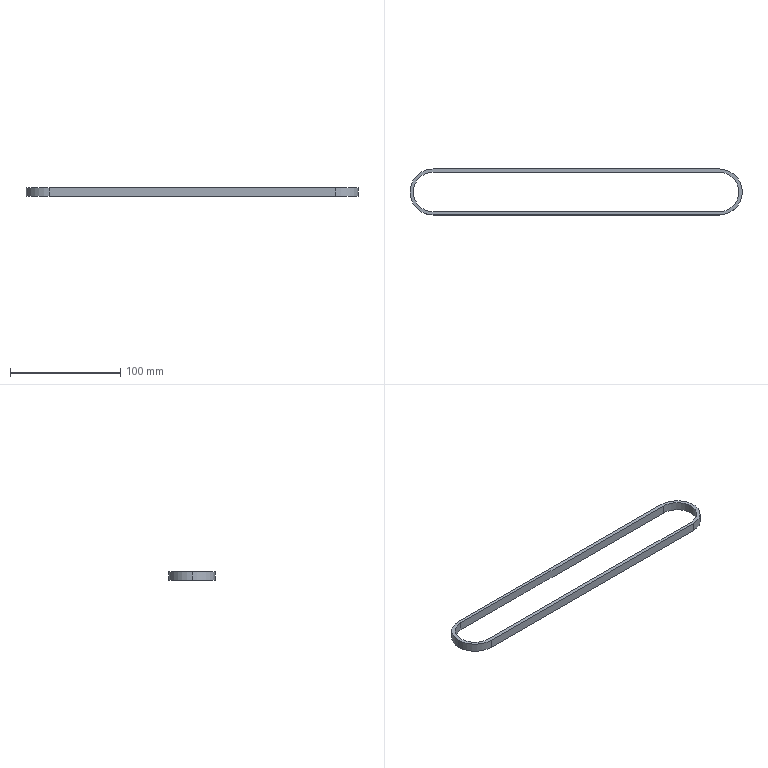Part | SolidWorks | features Extrusion 1, Shell 1 | 1 solid | 12 faces | box 301.8 x 41.8 x 7.9 mm | volume 15213 mm3 | cylinder 6 | plane 6 | commonest cylinder face diameters 35.8 x3 41.8 x3
STEP:
#1=CARTESIAN_POINT('',(-260.,17.9,7.9));
#2=VERTEX_POINT('',#1);
#3=CARTESIAN_POINT('',(-277.9,0.,7.9));
#4=VERTEX_POINT('',#3);
#5=CARTESIAN_POINT('',(-260.,0.,7.9));
#6=DIRECTION('',(0.,0.,1.));
#7=DIRECTION('',(1.,0.,0.));
#8=AXIS2_PLACEMENT_3D('',#5,#6,#7);
#9=CIRCLE('',#8,17.9);
#10=EDGE_CURVE('',#2,#4,#9,.T.);
#11=ORIENTED_EDGE('',*,*,#10,.T.);
#12=CARTESIAN_POINT('',(-277.9,0.,0.));
#13=VERTEX_POINT('',#12);
#14=CARTESIAN_POINT('',(-277.9,0.,7.9));
#15=DIRECTION('',(0.,0.,-1.));
#16=VECTOR('',#15,1000.);
#17=LINE('',#14,#16);
#18=EDGE_CURVE('',#4,#13,#17,.T.);
#19=ORIENTED_EDGE('',*,*,#18,.T.);
#20=CARTESIAN_POINT('',(-260.,17.9,0.));
#21=VERTEX_POINT('',#20);
#22=CARTESIAN_POINT('',(-260.,0.,0.));
#23=DIRECTION('',(0.,0.,1.));
#24=DIRECTION('',(1.,0.,0.));
#25=AXIS2_PLACEMENT_3D('',#22,#23,#24);
#26=CIRCLE('',#25,17.9);
#27=EDGE_CURVE('',#21,#13,#26,.T.);
#28=ORIENTED_EDGE('',*,*,#27,.F.);
#29=CARTESIAN_POINT('',(-260.,17.9,7.9));
#30=DIRECTION('',(0.,0.,-1.));
#31=VECTOR('',#30,1000.);
#32=LINE('',#29,#31);
#33=EDGE_CURVE('',#2,#21,#32,.T.);
#34=ORIENTED_EDGE('',*,*,#33,.F.);
#35=EDGE_LOOP('',(#11,#19,#28,#34));
#36=FACE_OUTER_BOUND('',#35,.T.);
#37=CARTESIAN_POINT('',(-260.,0.,7.9));
#38=DIRECTION('',(0.,0.,-1.));
#39=DIRECTION('',(-1.,0.,0.));
#40=AXIS2_PLACEMENT_3D('',#37,#38,#39);
#41=CYLINDRICAL_SURFACE('',#40,17.9);
#42=ADVANCED_FACE('',(#36),#41,.F.);
#43=CARTESIAN_POINT('',(-280.9,0.,7.9));
#44=VERTEX_POINT('',#43);
#45=CARTESIAN_POINT('',(-260.,-20.9,7.9));
#46=VERTEX_POINT('',#45);
#47=CARTESIAN_POINT('',(-260.,0.,7.9));
#48=DIRECTION('',(0.,0.,1.));
#49=DIRECTION('',(1.,0.,0.));
#50=AXIS2_PLACEMENT_3D('',#47,#48,#49);
#51=CIRCLE('',#50,20.9);
#52=EDGE_CURVE('',#44,#46,#51,.T.);
#53=ORIENTED_EDGE('',*,*,#52,.F.);
#54=CARTESIAN_POINT('',(-280.9,0.,0.));
#55=VERTEX_POINT('',#54);
#56=CARTESIAN_POINT('',(-280.9,0.,7.9));
#57=DIRECTION('',(0.,0.,-1.));
#58=VECTOR('',#57,1000.);
#59=LINE('',#56,#58);
#60=EDGE_CURVE('',#44,#55,#59,.T.);
#61=ORIENTED_EDGE('',*,*,#60,.T.);
#62=CARTESIAN_POINT('',(-260.,-20.9,0.));
#63=VERTEX_POINT('',#62);
#64=CARTESIAN_POINT('',(-260.,0.,0.));
#65=DIRECTION('',(0.,0.,1.));
#66=DIRECTION('',(1.,0.,0.));
#67=AXIS2_PLACEMENT_3D('',#64,#65,#66);
#68=CIRCLE('',#67,20.9);
#69=EDGE_CURVE('',#55,#63,#68,.T.);
#70=ORIENTED_EDGE('',*,*,#69,.T.);
#71=CARTESIAN_POINT('',(-260.,-20.9,7.9));
#72=DIRECTION('',(0.,0.,-1.));
#73=VECTOR('',#72,1000.);
#74=LINE('',#71,#73);
#75=EDGE_CURVE('',#46,#63,#74,.T.);
#76=ORIENTED_EDGE('',*,*,#75,.F.);
#77=EDGE_LOOP('',(#53,#61,#70,#76));
#78=FACE_OUTER_BOUND('',#77,.T.);
#79=CARTESIAN_POINT('',(-260.,0.,7.9));
#80=DIRECTION('',(0.,0.,-1.));
#81=DIRECTION('',(-1.,0.,0.));
#82=AXIS2_PLACEMENT_3D('',#79,#80,#81);
#83=CYLINDRICAL_SURFACE('',#82,20.9);
#84=ADVANCED_FACE('',(#78),#83,.T.);
#85=CARTESIAN_POINT('',(0.,-20.9,0.));
#86=VERTEX_POINT('',#85);
#87=CARTESIAN_POINT('',(0.,20.9,0.));
#88=VERTEX_POINT('',#87);
#89=CARTESIAN_POINT('',(0.,0.,0.));
#90=DIRECTION('',(0.,0.,1.));
#91=DIRECTION('',(1.,0.,0.));
#92=AXIS2_PLACEMENT_3D('',#89,#90,#91);
#93=CIRCLE('',#92,20.9);
#94=EDGE_CURVE('',#86,#88,#93,.T.);
#95=ORIENTED_EDGE('',*,*,#94,.T.);
#96=CARTESIAN_POINT('',(0.,20.9,7.9));
#97=VERTEX_POINT('',#96);
#98=CARTESIAN_POINT('',(0.,20.9,7.9));
#99=DIRECTION('',(0.,0.,-1.));
#100=VECTOR('',#99,1000.);
#101=LINE('',#98,#100);
#102=EDGE_CURVE('',#97,#88,#101,.T.);
#103=ORIENTED_EDGE('',*,*,#102,.F.);
#104=CARTESIAN_POINT('',(0.,-20.9,7.9));
#105=VERTEX_POINT('',#104);
#106=CARTESIAN_POINT('',(0.,0.,7.9));
#107=DIRECTION('',(0.,0.,1.));
#108=DIRECTION('',(1.,0.,0.));
#109=AXIS2_PLACEMENT_3D('',#106,#107,#108);
#110=CIRCLE('',#109,20.9);
#111=EDGE_CURVE('',#105,#97,#110,.T.);
#112=ORIENTED_EDGE('',*,*,#111,.F.);
#113=CARTESIAN_POINT('',(0.,-20.9,7.9));
#114=DIRECTION('',(0.,0.,-1.));
#115=VECTOR('',#114,1000.);
#116=LINE('',#113,#115);
#117=EDGE_CURVE('',#105,#86,#116,.T.);
#118=ORIENTED_EDGE('',*,*,#117,.T.);
#119=EDGE_LOOP('',(#95,#103,#112,#118));
#120=FACE_OUTER_BOUND('',#119,.T.);
#121=CARTESIAN_POINT('',(0.,0.,7.9));
#122=DIRECTION('',(0.,0.,-1.));
#123=DIRECTION('',(-1.,0.,0.));
#124=AXIS2_PLACEMENT_3D('',#121,#122,#123);
#125=CYLINDRICAL_SURFACE('',#124,20.9);
#126=ADVANCED_FACE('',(#120),#125,.T.);
#127=CARTESIAN_POINT('',(-260.,20.9,0.));
#128=VERTEX_POINT('',#127);
#129=CARTESIAN_POINT('',(0.,20.9,0.));
#130=DIRECTION('',(-1.,0.,0.));
#131=VECTOR('',#130,1000.);
#132=LINE('',#129,#131);
#133=EDGE_CURVE('',#88,#128,#132,.T.);
#134=ORIENTED_EDGE('',*,*,#133,.T.);
#135=CARTESIAN_POINT('',(-260.,20.9,7.9));
#136=VERTEX_POINT('',#135);
#137=CARTESIAN_POINT('',(-260.,20.9,7.9));
#138=DIRECTION('',(0.,0.,-1.));
#139=VECTOR('',#138,1000.);
#140=LINE('',#137,#139);
#141=EDGE_CURVE('',#136,#128,#140,.T.);
#142=ORIENTED_EDGE('',*,*,#141,.F.);
#143=CARTESIAN_POINT('',(0.,20.9,7.9));
#144=DIRECTION('',(-1.,0.,0.));
#145=VECTOR('',#144,1000.);
#146=LINE('',#143,#145);
#147=EDGE_CURVE('',#97,#136,#146,.T.);
#148=ORIENTED_EDGE('',*,*,#147,.F.);
#149=ORIENTED_EDGE('',*,*,#102,.T.);
#150=EDGE_LOOP('',(#134,#142,#148,#149));
#151=FACE_OUTER_BOUND('',#150,.T.);
#152=CARTESIAN_POINT('',(0.,20.9,7.9));
#153=DIRECTION('',(0.,-1.,0.));
#154=DIRECTION('',(0.,0.,-1.));
#155=AXIS2_PLACEMENT_3D('',#152,#153,#154);
#156=PLANE('',#155);
#157=ADVANCED_FACE('',(#151),#156,.F.);
#158=ORIENTED_EDGE('',*,*,#60,.F.);
#159=CARTESIAN_POINT('',(-260.,0.,7.9));
#160=DIRECTION('',(0.,0.,1.));
#161=DIRECTION('',(1.,0.,0.));
#162=AXIS2_PLACEMENT_3D('',#159,#160,#161);
#163=CIRCLE('',#162,20.9);
#164=EDGE_CURVE('',#136,#44,#163,.T.);
#165=ORIENTED_EDGE('',*,*,#164,.F.);
#166=ORIENTED_EDGE('',*,*,#141,.T.);
#167=CARTESIAN_POINT('',(-260.,0.,0.));
#168=DIRECTION('',(0.,0.,1.));
#169=DIRECTION('',(1.,0.,0.));
#170=AXIS2_PLACEMENT_3D('',#167,#168,#169);
#171=CIRCLE('',#170,20.9);
#172=EDGE_CURVE('',#128,#55,#171,.T.);
#173=ORIENTED_EDGE('',*,*,#172,.T.);
#174=EDGE_LOOP('',(#158,#165,#166,#173));
#175=FACE_OUTER_BOUND('',#174,.T.);
#176=CARTESIAN_POINT('',(-260.,0.,7.9));
#177=DIRECTION('',(0.,0.,-1.));
#178=DIRECTION('',(-1.,0.,0.));
#179=AXIS2_PLACEMENT_3D('',#176,#177,#178);
#180=CYLINDRICAL_SURFACE('',#179,20.9);
#181=ADVANCED_FACE('',(#175),#180,.T.);
#182=CARTESIAN_POINT('',(0.,-20.9,0.));
#183=DIRECTION('',(1.,0.,0.));
#184=VECTOR('',#183,1000.);
#185=LINE('',#182,#184);
#186=EDGE_CURVE('',#63,#86,#185,.T.);
#187=ORIENTED_EDGE('',*,*,#186,.T.);
#188=ORIENTED_EDGE('',*,*,#117,.F.);
#189=CARTESIAN_POINT('',(0.,-20.9,7.9));
#190=DIRECTION('',(1.,0.,0.));
#191=VECTOR('',#190,1000.);
#192=LINE('',#189,#191);
#193=EDGE_CURVE('',#46,#105,#192,.T.);
#194=ORIENTED_EDGE('',*,*,#193,.F.);
#195=ORIENTED_EDGE('',*,*,#75,.T.);
#196=EDGE_LOOP('',(#187,#188,#194,#195));
#197=FACE_OUTER_BOUND('',#196,.T.);
#198=CARTESIAN_POINT('',(0.,-20.9,7.9));
#199=DIRECTION('',(0.,1.,0.));
#200=DIRECTION('',(0.,0.,1.));
#201=AXIS2_PLACEMENT_3D('',#198,#199,#200);
#202=PLANE('',#201);
#203=ADVANCED_FACE('',(#197),#202,.F.);
#204=CARTESIAN_POINT('',(0.,-17.9,7.9));
#205=VERTEX_POINT('',#204);
#206=CARTESIAN_POINT('',(0.,17.9,7.9));
#207=VERTEX_POINT('',#206);
#208=CARTESIAN_POINT('',(0.,0.,7.9));
#209=DIRECTION('',(0.,0.,1.));
#210=DIRECTION('',(1.,0.,0.));
#211=AXIS2_PLACEMENT_3D('',#208,#209,#210);
#212=CIRCLE('',#211,17.9);
#213=EDGE_CURVE('',#205,#207,#212,.T.);
#214=ORIENTED_EDGE('',*,*,#213,.F.);
#215=CARTESIAN_POINT('',(-260.,-17.9,7.9));
#216=VERTEX_POINT('',#215);
#217=CARTESIAN_POINT('',(0.,-17.9,7.9));
#218=DIRECTION('',(1.,0.,0.));
#219=VECTOR('',#218,1000.);
#220=LINE('',#217,#219);
#221=EDGE_CURVE('',#216,#205,#220,.T.);
#222=ORIENTED_EDGE('',*,*,#221,.F.);
#223=CARTESIAN_POINT('',(-260.,0.,7.9));
#224=DIRECTION('',(0.,0.,1.));
#225=DIRECTION('',(1.,0.,0.));
#226=AXIS2_PLACEMENT_3D('',#223,#224,#225);
#227=CIRCLE('',#226,17.9);
#228=EDGE_CURVE('',#4,#216,#227,.T.);
#229=ORIENTED_EDGE('',*,*,#228,.F.);
#230=ORIENTED_EDGE('',*,*,#10,.F.);
#231=CARTESIAN_POINT('',(0.,17.9,7.9));
#232=DIRECTION('',(-1.,0.,0.));
#233=VECTOR('',#232,1000.);
#234=LINE('',#231,#233);
#235=EDGE_CURVE('',#207,#2,#234,.T.);
#236=ORIENTED_EDGE('',*,*,#235,.F.);
#237=EDGE_LOOP('',(#214,#222,#229,#230,#236));
#238=FACE_BOUND('',#237,.T.);
#239=ORIENTED_EDGE('',*,*,#111,.T.);
#240=ORIENTED_EDGE('',*,*,#147,.T.);
#241=ORIENTED_EDGE('',*,*,#164,.T.);
#242=ORIENTED_EDGE('',*,*,#52,.T.);
#243=ORIENTED_EDGE('',*,*,#193,.T.);
#244=EDGE_LOOP('',(#239,#240,#241,#242,#243));
#245=FACE_OUTER_BOUND('',#244,.T.);
#246=CARTESIAN_POINT('',(0.,0.,7.9));
#247=DIRECTION('',(0.,0.,1.));
#248=DIRECTION('',(1.,0.,0.));
#249=AXIS2_PLACEMENT_3D('',#246,#247,#248);
#250=PLANE('',#249);
#251=ADVANCED_FACE('',(#238,#245),#250,.T.);
#252=CARTESIAN_POINT('',(-260.,-17.9,0.));
#253=VERTEX_POINT('',#252);
#254=CARTESIAN_POINT('',(0.,-17.9,0.));
#255=VERTEX_POINT('',#254);
#256=CARTESIAN_POINT('',(0.,-17.9,0.));
#257=DIRECTION('',(1.,0.,0.));
#258=VECTOR('',#257,1000.);
#259=LINE('',#256,#258);
#260=EDGE_CURVE('',#253,#255,#259,.T.);
#261=ORIENTED_EDGE('',*,*,#260,.T.);
#262=CARTESIAN_POINT('',(0.,17.9,0.));
#263=VERTEX_POINT('',#262);
#264=CARTESIAN_POINT('',(0.,0.,0.));
#265=DIRECTION('',(0.,0.,1.));
#266=DIRECTION('',(1.,0.,0.));
#267=AXIS2_PLACEMENT_3D('',#264,#265,#266);
#268=CIRCLE('',#267,17.9);
#269=EDGE_CURVE('',#255,#263,#268,.T.);
#270=ORIENTED_EDGE('',*,*,#269,.T.);
#271=CARTESIAN_POINT('',(0.,17.9,0.));
#272=DIRECTION('',(-1.,0.,0.));
#273=VECTOR('',#272,1000.);
#274=LINE('',#271,#273);
#275=EDGE_CURVE('',#263,#21,#274,.T.);
#276=ORIENTED_EDGE('',*,*,#275,.T.);
#277=ORIENTED_EDGE('',*,*,#27,.T.);
#278=CARTESIAN_POINT('',(-260.,0.,0.));
#279=DIRECTION('',(0.,0.,1.));
#280=DIRECTION('',(1.,0.,0.));
#281=AXIS2_PLACEMENT_3D('',#278,#279,#280);
#282=CIRCLE('',#281,17.9);
#283=EDGE_CURVE('',#13,#253,#282,.T.);
#284=ORIENTED_EDGE('',*,*,#283,.T.);
#285=EDGE_LOOP('',(#261,#270,#276,#277,#284));
#286=FACE_BOUND('',#285,.T.);
#287=ORIENTED_EDGE('',*,*,#94,.F.);
#288=ORIENTED_EDGE('',*,*,#186,.F.);
#289=ORIENTED_EDGE('',*,*,#69,.F.);
#290=ORIENTED_EDGE('',*,*,#172,.F.);
#291=ORIENTED_EDGE('',*,*,#133,.F.);
#292=EDGE_LOOP('',(#287,#288,#289,#290,#291));
#293=FACE_OUTER_BOUND('',#292,.T.);
#294=CARTESIAN_POINT('',(0.,0.,0.));
#295=DIRECTION('',(0.,0.,1.));
#296=DIRECTION('',(1.,0.,0.));
#297=AXIS2_PLACEMENT_3D('',#294,#295,#296);
#298=PLANE('',#297);
#299=ADVANCED_FACE('',(#286,#293),#298,.F.);
#300=ORIENTED_EDGE('',*,*,#269,.F.);
#301=CARTESIAN_POINT('',(0.,-17.9,7.9));
#302=DIRECTION('',(0.,0.,-1.));
#303=VECTOR('',#302,1000.);
#304=LINE('',#301,#303);
#305=EDGE_CURVE('',#205,#255,#304,.T.);
#306=ORIENTED_EDGE('',*,*,#305,.F.);
#307=ORIENTED_EDGE('',*,*,#213,.T.);
#308=CARTESIAN_POINT('',(0.,17.9,7.9));
#309=DIRECTION('',(0.,0.,-1.));
#310=VECTOR('',#309,1000.);
#311=LINE('',#308,#310);
#312=EDGE_CURVE('',#207,#263,#311,.T.);
#313=ORIENTED_EDGE('',*,*,#312,.T.);
#314=EDGE_LOOP('',(#300,#306,#307,#313));
#315=FACE_OUTER_BOUND('',#314,.T.);
#316=CARTESIAN_POINT('',(0.,0.,7.9));
#317=DIRECTION('',(0.,0.,-1.));
#318=DIRECTION('',(-1.,0.,0.));
#319=AXIS2_PLACEMENT_3D('',#316,#317,#318);
#320=CYLINDRICAL_SURFACE('',#319,17.9);
#321=ADVANCED_FACE('',(#315),#320,.F.);
#322=ORIENTED_EDGE('',*,*,#275,.F.);
#323=ORIENTED_EDGE('',*,*,#312,.F.);
#324=ORIENTED_EDGE('',*,*,#235,.T.);
#325=ORIENTED_EDGE('',*,*,#33,.T.);
#326=EDGE_LOOP('',(#322,#323,#324,#325));
#327=FACE_OUTER_BOUND('',#326,.T.);
#328=CARTESIAN_POINT('',(0.,17.9,7.9));
#329=DIRECTION('',(0.,-1.,0.));
#330=DIRECTION('',(0.,0.,-1.));
#331=AXIS2_PLACEMENT_3D('',#328,#329,#330);
#332=PLANE('',#331);
#333=ADVANCED_FACE('',(#327),#332,.T.);
#334=ORIENTED_EDGE('',*,*,#18,.F.);
#335=ORIENTED_EDGE('',*,*,#228,.T.);
#336=CARTESIAN_POINT('',(-260.,-17.9,7.9));
#337=DIRECTION('',(0.,0.,-1.));
#338=VECTOR('',#337,1000.);
#339=LINE('',#336,#338);
#340=EDGE_CURVE('',#216,#253,#339,.T.);
#341=ORIENTED_EDGE('',*,*,#340,.T.);
#342=ORIENTED_EDGE('',*,*,#283,.F.);
#343=EDGE_LOOP('',(#334,#335,#341,#342));
#344=FACE_OUTER_BOUND('',#343,.T.);
#345=CARTESIAN_POINT('',(-260.,0.,7.9));
#346=DIRECTION('',(0.,0.,-1.));
#347=DIRECTION('',(-1.,0.,0.));
#348=AXIS2_PLACEMENT_3D('',#345,#346,#347);
#349=CYLINDRICAL_SURFACE('',#348,17.9);
#350=ADVANCED_FACE('',(#344),#349,.F.);
#351=ORIENTED_EDGE('',*,*,#260,.F.);
#352=ORIENTED_EDGE('',*,*,#340,.F.);
#353=ORIENTED_EDGE('',*,*,#221,.T.);
#354=ORIENTED_EDGE('',*,*,#305,.T.);
#355=EDGE_LOOP('',(#351,#352,#353,#354));
#356=FACE_OUTER_BOUND('',#355,.T.);
#357=CARTESIAN_POINT('',(0.,-17.9,7.9));
#358=DIRECTION('',(0.,1.,0.));
#359=DIRECTION('',(0.,0.,1.));
#360=AXIS2_PLACEMENT_3D('',#357,#358,#359);
#361=PLANE('',#360);
#362=ADVANCED_FACE('',(#356),#361,.T.);
#363=CLOSED_SHELL('',(#42,#84,#126,#157,#181,#203,#251,#299,#321,#333,#350,#362));
#364=MANIFOLD_SOLID_BREP('',#363);
#365=CARTESIAN_POINT('',(0.,0.,0.));
#366=DIRECTION('',(0.,0.,1.));
#367=DIRECTION('',(1.,0.,0.));
#368=AXIS2_PLACEMENT_3D('',#365,#366,#367);
#369=(LENGTH_UNIT()NAMED_UNIT(*)SI_UNIT(.MILLI.,.METRE.));
#370=UNCERTAINTY_MEASURE_WITH_UNIT(LENGTH_MEASURE(0.00001),#369,'','');
#371=(NAMED_UNIT(*)PLANE_ANGLE_UNIT()SI_UNIT($,.RADIAN.));
#372=(NAMED_UNIT(*)SI_UNIT($,.STERADIAN.)SOLID_ANGLE_UNIT());
#373=(GEOMETRIC_REPRESENTATION_CONTEXT(3)GLOBAL_UNCERTAINTY_ASSIGNED_CONTEXT((#370))GLOBAL_UNIT_ASSIGNED_CONTEXT((#369,#371,#372))REPRESENTATION_CONTEXT('',''));
#374=ADVANCED_BREP_SHAPE_REPRESENTATION('',(#364,#368),#373);